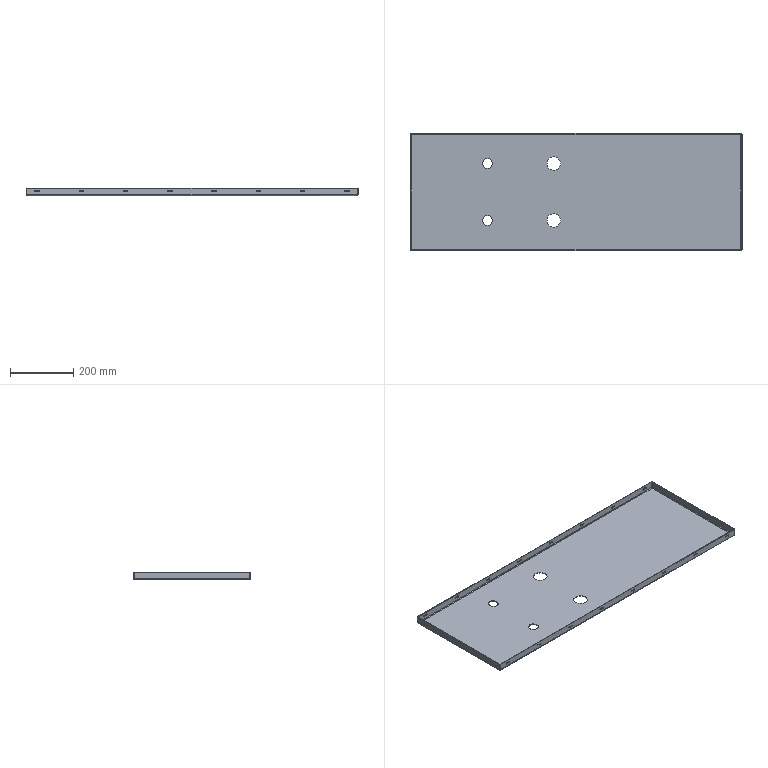Part | SolidWorks | features ICE 2, Cut 1, EdgeFlange 1, FlatPattern 1, LPattern 1, SMBaseFlange 1, SheetMetal 1 | 1 solid | 110 faces | box 1050 x 370 x 25 mm | volume 888515 mm3 | plane 54 | cylinder 48 | spline 8 | commonest cylinder face diameters 4.5 x32 4 x4 8 x4 31 x4 43 x4